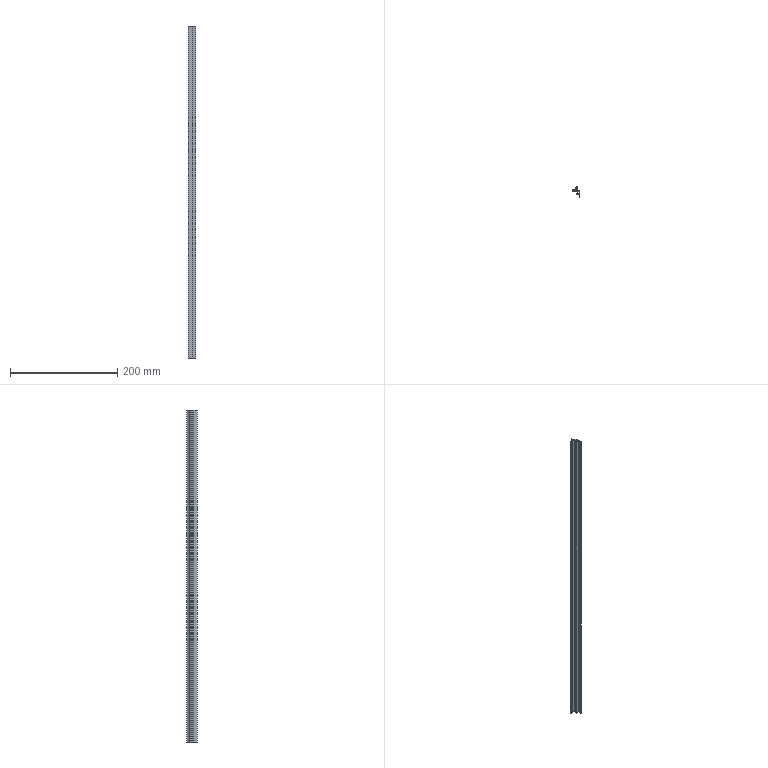Part | SolidWorks | features BaseBody 1, ICE 1, MoveFace 1 | 1 solid | 27 faces | box 14 x 20.3 x 620 mm | volume 31568 mm3 | plane 20 | cylinder 7 | commonest cylinder face diameters 0.387 x2 0.8 x2 0.4 x1 20 x1 22 x1
STEP:
#1=CARTESIAN_POINT('',(-5.304,-0.625,200.));
#2=VERTEX_POINT('',#1);
#3=CARTESIAN_POINT('',(-5.449,-0.8125,200.));
#4=VERTEX_POINT('',#3);
#5=CARTESIAN_POINT('',(-5.255,-0.8125,200.));
#6=DIRECTION('',(0.,0.,1.));
#7=DIRECTION('',(-1.,0.,0.));
#8=AXIS2_PLACEMENT_3D('',#5,#6,#7);
#9=CIRCLE('',#8,0.1937);
#10=EDGE_CURVE('',#2,#4,#9,.T.);
#11=ORIENTED_EDGE('',*,*,#10,.T.);
#12=CARTESIAN_POINT('',(-5.449,-0.8125,-420.));
#13=VERTEX_POINT('',#12);
#14=CARTESIAN_POINT('',(-5.449,-0.8125,230.));
#15=DIRECTION('',(0.,0.,-1.));
#16=VECTOR('',#15,1000.);
#17=LINE('',#14,#16);
#18=EDGE_CURVE('',#4,#13,#17,.T.);
#19=ORIENTED_EDGE('',*,*,#18,.T.);
#20=CARTESIAN_POINT('',(-5.304,-0.625,-420.));
#21=VERTEX_POINT('',#20);
#22=CARTESIAN_POINT('',(-5.255,-0.8125,-420.));
#23=DIRECTION('',(0.,0.,-1.));
#24=DIRECTION('',(1.,0.,0.));
#25=AXIS2_PLACEMENT_3D('',#22,#23,#24);
#26=CIRCLE('',#25,0.1937);
#27=EDGE_CURVE('',#13,#21,#26,.T.);
#28=ORIENTED_EDGE('',*,*,#27,.T.);
#29=CARTESIAN_POINT('',(-5.304,-0.625,230.));
#30=DIRECTION('',(0.,0.,-1.));
#31=VECTOR('',#30,1000.);
#32=LINE('',#29,#31);
#33=EDGE_CURVE('',#2,#21,#32,.T.);
#34=ORIENTED_EDGE('',*,*,#33,.F.);
#35=EDGE_LOOP('',(#11,#19,#28,#34));
#36=FACE_OUTER_BOUND('',#35,.T.);
#37=CARTESIAN_POINT('',(-5.255,-0.8125,230.));
#38=DIRECTION('',(0.,0.,-1.));
#39=DIRECTION('',(-1.,0.,0.));
#40=AXIS2_PLACEMENT_3D('',#37,#38,#39);
#41=CYLINDRICAL_SURFACE('',#40,0.1937);
#42=ADVANCED_FACE('',(#36),#41,.F.);
#43=CARTESIAN_POINT('',(5.,-1.,-420.));
#44=VERTEX_POINT('',#43);
#45=CARTESIAN_POINT('',(5.,-14.3,-420.));
#46=VERTEX_POINT('',#45);
#47=CARTESIAN_POINT('',(5.,29.623,-420.));
#48=DIRECTION('',(0.,-1.,0.));
#49=VECTOR('',#48,1000.);
#50=LINE('',#47,#49);
#51=EDGE_CURVE('',#44,#46,#50,.T.);
#52=ORIENTED_EDGE('',*,*,#51,.F.);
#53=CARTESIAN_POINT('',(5.,-1.,200.));
#54=VERTEX_POINT('',#53);
#55=CARTESIAN_POINT('',(5.,-1.,230.));
#56=DIRECTION('',(0.,0.,-1.));
#57=VECTOR('',#56,1000.);
#58=LINE('',#55,#57);
#59=EDGE_CURVE('',#54,#44,#58,.T.);
#60=ORIENTED_EDGE('',*,*,#59,.F.);
#61=CARTESIAN_POINT('',(5.,-14.3,200.));
#62=VERTEX_POINT('',#61);
#63=CARTESIAN_POINT('',(5.,-14.3,200.));
#64=DIRECTION('',(0.,1.,0.));
#65=VECTOR('',#64,1000.);
#66=LINE('',#63,#65);
#67=EDGE_CURVE('',#62,#54,#66,.T.);
#68=ORIENTED_EDGE('',*,*,#67,.F.);
#69=CARTESIAN_POINT('',(5.,-14.3,230.));
#70=DIRECTION('',(0.,0.,1.));
#71=VECTOR('',#70,1000.);
#72=LINE('',#69,#71);
#73=EDGE_CURVE('',#46,#62,#72,.T.);
#74=ORIENTED_EDGE('',*,*,#73,.F.);
#75=EDGE_LOOP('',(#52,#60,#68,#74));
#76=FACE_OUTER_BOUND('',#75,.T.);
#77=CARTESIAN_POINT('',(5.,-14.3,230.));
#78=DIRECTION('',(-1.,0.,0.));
#79=DIRECTION('',(0.,0.,1.));
#80=AXIS2_PLACEMENT_3D('',#77,#78,#79);
#81=PLANE('',#80);
#82=ADVANCED_FACE('',(#76),#81,.F.);
#83=CARTESIAN_POINT('',(-9.,-2.,-420.));
#84=VERTEX_POINT('',#83);
#85=CARTESIAN_POINT('',(-9.,-2.,200.));
#86=VERTEX_POINT('',#85);
#87=CARTESIAN_POINT('',(-9.,-2.,230.));
#88=DIRECTION('',(0.,0.,1.));
#89=VECTOR('',#88,1000.);
#90=LINE('',#87,#89);
#91=EDGE_CURVE('',#84,#86,#90,.T.);
#92=ORIENTED_EDGE('',*,*,#91,.F.);
#93=CARTESIAN_POINT('',(0.9,-2.,-420.));
#94=VERTEX_POINT('',#93);
#95=CARTESIAN_POINT('',(5.,-2.,-420.));
#96=DIRECTION('',(-1.,0.,0.));
#97=VECTOR('',#96,1000.);
#98=LINE('',#95,#97);
#99=EDGE_CURVE('',#94,#84,#98,.T.);
#100=ORIENTED_EDGE('',*,*,#99,.F.);
#101=CARTESIAN_POINT('',(0.9,-2.,200.));
#102=VERTEX_POINT('',#101);
#103=CARTESIAN_POINT('',(0.9,-2.,230.));
#104=DIRECTION('',(0.,0.,-1.));
#105=VECTOR('',#104,1000.);
#106=LINE('',#103,#105);
#107=EDGE_CURVE('',#102,#94,#106,.T.);
#108=ORIENTED_EDGE('',*,*,#107,.F.);
#109=CARTESIAN_POINT('',(5.,-2.,200.));
#110=DIRECTION('',(1.,0.,0.));
#111=VECTOR('',#110,1000.);
#112=LINE('',#109,#111);
#113=EDGE_CURVE('',#86,#102,#112,.T.);
#114=ORIENTED_EDGE('',*,*,#113,.F.);
#115=EDGE_LOOP('',(#92,#100,#108,#114));
#116=FACE_OUTER_BOUND('',#115,.T.);
#117=CARTESIAN_POINT('',(-9.,-2.,230.));
#118=DIRECTION('',(0.,1.,0.));
#119=DIRECTION('',(0.,0.,1.));
#120=AXIS2_PLACEMENT_3D('',#117,#118,#119);
#121=PLANE('',#120);
#122=ADVANCED_FACE('',(#116),#121,.F.);
#123=CARTESIAN_POINT('',(4.,-6.,200.));
#124=VERTEX_POINT('',#123);
#125=CARTESIAN_POINT('',(4.,-3.,200.));
#126=VERTEX_POINT('',#125);
#127=CARTESIAN_POINT('',(4.,29.623,200.));
#128=DIRECTION('',(0.,1.,0.));
#129=VECTOR('',#128,1000.);
#130=LINE('',#127,#129);
#131=EDGE_CURVE('',#124,#126,#130,.T.);
#132=ORIENTED_EDGE('',*,*,#131,.F.);
#133=CARTESIAN_POINT('',(1.,-6.,200.));
#134=VERTEX_POINT('',#133);
#135=CARTESIAN_POINT('',(5.,-6.,200.));
#136=DIRECTION('',(1.,0.,0.));
#137=VECTOR('',#136,1000.);
#138=LINE('',#135,#137);
#139=EDGE_CURVE('',#134,#124,#138,.T.);
#140=ORIENTED_EDGE('',*,*,#139,.F.);
#141=CARTESIAN_POINT('',(1.,-6.7,200.));
#142=VERTEX_POINT('',#141);
#143=CARTESIAN_POINT('',(1.,-6.,200.));
#144=DIRECTION('',(0.,-1.,0.));
#145=VECTOR('',#144,1000.);
#146=LINE('',#143,#145);
#147=EDGE_CURVE('',#134,#142,#146,.T.);
#148=ORIENTED_EDGE('',*,*,#147,.T.);
#149=CARTESIAN_POINT('',(-1.7,-6.7,200.));
#150=VERTEX_POINT('',#149);
#151=CARTESIAN_POINT('',(5.,-6.7,200.));
#152=DIRECTION('',(1.,0.,0.));
#153=VECTOR('',#152,1000.);
#154=LINE('',#151,#153);
#155=EDGE_CURVE('',#150,#142,#154,.T.);
#156=ORIENTED_EDGE('',*,*,#155,.F.);
#157=CARTESIAN_POINT('',(-1.7,-7.7,200.));
#158=VERTEX_POINT('',#157);
#159=CARTESIAN_POINT('',(-1.7,-6.7,200.));
#160=DIRECTION('',(0.,-1.,0.));
#161=VECTOR('',#160,1000.);
#162=LINE('',#159,#161);
#163=EDGE_CURVE('',#150,#158,#162,.T.);
#164=ORIENTED_EDGE('',*,*,#163,.T.);
#165=CARTESIAN_POINT('',(4.,-7.7,200.));
#166=VERTEX_POINT('',#165);
#167=CARTESIAN_POINT('',(5.,-7.7,200.));
#168=DIRECTION('',(-1.,0.,0.));
#169=VECTOR('',#168,1000.);
#170=LINE('',#167,#169);
#171=EDGE_CURVE('',#166,#158,#170,.T.);
#172=ORIENTED_EDGE('',*,*,#171,.F.);
#173=CARTESIAN_POINT('',(4.,-14.3,200.));
#174=VERTEX_POINT('',#173);
#175=CARTESIAN_POINT('',(4.,29.623,200.));
#176=DIRECTION('',(0.,1.,0.));
#177=VECTOR('',#176,1000.);
#178=LINE('',#175,#177);
#179=EDGE_CURVE('',#174,#166,#178,.T.);
#180=ORIENTED_EDGE('',*,*,#179,.F.);
#181=CARTESIAN_POINT('',(5.,-14.3,200.));
#182=DIRECTION('',(-1.,0.,0.));
#183=VECTOR('',#182,1000.);
#184=LINE('',#181,#183);
#185=EDGE_CURVE('',#62,#174,#184,.T.);
#186=ORIENTED_EDGE('',*,*,#185,.F.);
#187=ORIENTED_EDGE('',*,*,#67,.T.);
#188=CARTESIAN_POINT('',(-5.207,-1.,200.));
#189=VERTEX_POINT('',#188);
#190=CARTESIAN_POINT('',(5.,-1.,200.));
#191=DIRECTION('',(1.,0.,0.));
#192=VECTOR('',#191,1000.);
#193=LINE('',#190,#192);
#194=EDGE_CURVE('',#189,#54,#193,.T.);
#195=ORIENTED_EDGE('',*,*,#194,.F.);
#196=CARTESIAN_POINT('',(-5.255,-0.8125,200.));
#197=DIRECTION('',(0.,0.,1.));
#198=DIRECTION('',(-1.,0.,0.));
#199=AXIS2_PLACEMENT_3D('',#196,#197,#198);
#200=CIRCLE('',#199,0.1937);
#201=EDGE_CURVE('',#4,#189,#200,.T.);
#202=ORIENTED_EDGE('',*,*,#201,.F.);
#203=ORIENTED_EDGE('',*,*,#10,.F.);
#204=CARTESIAN_POINT('',(-1.368,3.063,200.));
#205=VERTEX_POINT('',#204);
#206=CARTESIAN_POINT('',(-10.628,9.,200.));
#207=DIRECTION('',(0.,0.,1.));
#208=DIRECTION('',(-1.,0.,0.));
#209=AXIS2_PLACEMENT_3D('',#206,#207,#208);
#210=CIRCLE('',#209,11.);
#211=EDGE_CURVE('',#2,#205,#210,.T.);
#212=ORIENTED_EDGE('',*,*,#211,.T.);
#213=CARTESIAN_POINT('',(-1.,2.955,200.));
#214=VERTEX_POINT('',#213);
#215=CARTESIAN_POINT('',(-1.2,2.955,200.));
#216=DIRECTION('',(0.,0.,1.));
#217=DIRECTION('',(-1.,0.,0.));
#218=AXIS2_PLACEMENT_3D('',#215,#216,#217);
#219=CIRCLE('',#218,0.2);
#220=EDGE_CURVE('',#214,#205,#219,.T.);
#221=ORIENTED_EDGE('',*,*,#220,.F.);
#222=CARTESIAN_POINT('',(-1.,1.5,200.));
#223=VERTEX_POINT('',#222);
#224=CARTESIAN_POINT('',(-1.,2.955,200.));
#225=DIRECTION('',(0.,1.,0.));
#226=VECTOR('',#225,1000.);
#227=LINE('',#224,#226);
#228=EDGE_CURVE('',#223,#214,#227,.T.);
#229=ORIENTED_EDGE('',*,*,#228,.F.);
#230=CARTESIAN_POINT('',(0.,1.5,200.));
#231=VERTEX_POINT('',#230);
#232=CARTESIAN_POINT('',(-1.,1.5,200.));
#233=DIRECTION('',(-1.,0.,0.));
#234=VECTOR('',#233,1000.);
#235=LINE('',#232,#234);
#236=EDGE_CURVE('',#231,#223,#235,.T.);
#237=ORIENTED_EDGE('',*,*,#236,.F.);
#238=CARTESIAN_POINT('',(0.,6.,200.));
#239=VERTEX_POINT('',#238);
#240=CARTESIAN_POINT('',(0.,1.5,200.));
#241=DIRECTION('',(0.,-1.,0.));
#242=VECTOR('',#241,1000.);
#243=LINE('',#240,#242);
#244=EDGE_CURVE('',#239,#231,#243,.T.);
#245=ORIENTED_EDGE('',*,*,#244,.F.);
#246=CARTESIAN_POINT('',(-0.8,6.,200.));
#247=VERTEX_POINT('',#246);
#248=CARTESIAN_POINT('',(0.,6.,200.));
#249=DIRECTION('',(1.,0.,0.));
#250=VECTOR('',#249,1000.);
#251=LINE('',#248,#250);
#252=EDGE_CURVE('',#247,#239,#251,.T.);
#253=ORIENTED_EDGE('',*,*,#252,.F.);
#254=CARTESIAN_POINT('',(-1.178,5.731,200.));
#255=VERTEX_POINT('',#254);
#256=CARTESIAN_POINT('',(-0.8,5.6,200.));
#257=DIRECTION('',(0.,0.,1.));
#258=DIRECTION('',(-1.,0.,0.));
#259=AXIS2_PLACEMENT_3D('',#256,#257,#258);
#260=CIRCLE('',#259,0.4);
#261=EDGE_CURVE('',#247,#255,#260,.T.);
#262=ORIENTED_EDGE('',*,*,#261,.T.);
#263=CARTESIAN_POINT('',(-8.678,-0.8077,200.));
#264=VERTEX_POINT('',#263);
#265=CARTESIAN_POINT('',(-10.628,9.,200.));
#266=DIRECTION('',(0.,0.,1.));
#267=DIRECTION('',(-1.,0.,0.));
#268=AXIS2_PLACEMENT_3D('',#265,#266,#267);
#269=CIRCLE('',#268,10.);
#270=EDGE_CURVE('',#264,#255,#269,.T.);
#271=ORIENTED_EDGE('',*,*,#270,.F.);
#272=CARTESIAN_POINT('',(-9.,-1.2,200.));
#273=VERTEX_POINT('',#272);
#274=CARTESIAN_POINT('',(-8.6,-1.2,200.));
#275=DIRECTION('',(0.,0.,1.));
#276=DIRECTION('',(-1.,0.,0.));
#277=AXIS2_PLACEMENT_3D('',#274,#275,#276);
#278=CIRCLE('',#277,0.4);
#279=EDGE_CURVE('',#264,#273,#278,.T.);
#280=ORIENTED_EDGE('',*,*,#279,.T.);
#281=CARTESIAN_POINT('',(-9.,8.,200.));
#282=DIRECTION('',(0.,-1.,0.));
#283=VECTOR('',#282,1000.);
#284=LINE('',#281,#283);
#285=EDGE_CURVE('',#273,#86,#284,.T.);
#286=ORIENTED_EDGE('',*,*,#285,.T.);
#287=ORIENTED_EDGE('',*,*,#113,.T.);
#288=CARTESIAN_POINT('',(0.9,-3.,200.));
#289=VERTEX_POINT('',#288);
#290=CARTESIAN_POINT('',(0.9,29.623,200.));
#291=DIRECTION('',(0.,1.,0.));
#292=VECTOR('',#291,1000.);
#293=LINE('',#290,#292);
#294=EDGE_CURVE('',#289,#102,#293,.T.);
#295=ORIENTED_EDGE('',*,*,#294,.F.);
#296=CARTESIAN_POINT('',(5.,-3.,200.));
#297=DIRECTION('',(-1.,0.,0.));
#298=VECTOR('',#297,1000.);
#299=LINE('',#296,#298);
#300=EDGE_CURVE('',#126,#289,#299,.T.);
#301=ORIENTED_EDGE('',*,*,#300,.F.);
#302=EDGE_LOOP('',(#132,#140,#148,#156,#164,#172,#180,#186,#187,#195,#202,#203,#212,#221,#229,#237,#245,#253,#262,#271,#280,#286,#287,#295,#301));
#303=FACE_OUTER_BOUND('',#302,.T.);
#304=CARTESIAN_POINT('',(5.,29.623,200.));
#305=DIRECTION('',(0.,0.,-1.));
#306=DIRECTION('',(-1.,0.,0.));
#307=AXIS2_PLACEMENT_3D('',#304,#305,#306);
#308=PLANE('',#307);
#309=ADVANCED_FACE('',(#303),#308,.F.);
#310=ORIENTED_EDGE('',*,*,#185,.T.);
#311=CARTESIAN_POINT('',(4.,-14.3,-420.));
#312=VERTEX_POINT('',#311);
#313=CARTESIAN_POINT('',(4.,-14.3,230.));
#314=DIRECTION('',(0.,0.,1.));
#315=VECTOR('',#314,1000.);
#316=LINE('',#313,#315);
#317=EDGE_CURVE('',#312,#174,#316,.T.);
#318=ORIENTED_EDGE('',*,*,#317,.F.);
#319=CARTESIAN_POINT('',(5.,-14.3,-420.));
#320=DIRECTION('',(-1.,0.,0.));
#321=VECTOR('',#320,1000.);
#322=LINE('',#319,#321);
#323=EDGE_CURVE('',#46,#312,#322,.T.);
#324=ORIENTED_EDGE('',*,*,#323,.F.);
#325=ORIENTED_EDGE('',*,*,#73,.T.);
#326=EDGE_LOOP('',(#310,#318,#324,#325));
#327=FACE_OUTER_BOUND('',#326,.T.);
#328=CARTESIAN_POINT('',(4.,-14.3,230.));
#329=DIRECTION('',(0.,1.,0.));
#330=DIRECTION('',(0.,0.,1.));
#331=AXIS2_PLACEMENT_3D('',#328,#329,#330);
#332=PLANE('',#331);
#333=ADVANCED_FACE('',(#327),#332,.F.);
#334=ORIENTED_EDGE('',*,*,#51,.T.);
#335=ORIENTED_EDGE('',*,*,#323,.T.);
#336=CARTESIAN_POINT('',(4.,-7.7,-420.));
#337=VERTEX_POINT('',#336);
#338=CARTESIAN_POINT('',(4.,-7.7,-420.));
#339=DIRECTION('',(0.,-1.,0.));
#340=VECTOR('',#339,1000.);
#341=LINE('',#338,#340);
#342=EDGE_CURVE('',#337,#312,#341,.T.);
#343=ORIENTED_EDGE('',*,*,#342,.F.);
#344=CARTESIAN_POINT('',(-1.7,-7.7,-420.));
#345=VERTEX_POINT('',#344);
#346=CARTESIAN_POINT('',(-1.7,-7.7,-420.));
#347=DIRECTION('',(1.,0.,0.));
#348=VECTOR('',#347,1000.);
#349=LINE('',#346,#348);
#350=EDGE_CURVE('',#345,#337,#349,.T.);
#351=ORIENTED_EDGE('',*,*,#350,.F.);
#352=CARTESIAN_POINT('',(-1.7,-6.7,-420.));
#353=VERTEX_POINT('',#352);
#354=CARTESIAN_POINT('',(-1.7,29.623,-420.));
#355=DIRECTION('',(0.,1.,0.));
#356=VECTOR('',#355,1000.);
#357=LINE('',#354,#356);
#358=EDGE_CURVE('',#345,#353,#357,.T.);
#359=ORIENTED_EDGE('',*,*,#358,.T.);
#360=CARTESIAN_POINT('',(1.,-6.7,-420.));
#361=VERTEX_POINT('',#360);
#362=CARTESIAN_POINT('',(1.,-6.7,-420.));
#363=DIRECTION('',(-1.,0.,0.));
#364=VECTOR('',#363,1000.);
#365=LINE('',#362,#364);
#366=EDGE_CURVE('',#361,#353,#365,.T.);
#367=ORIENTED_EDGE('',*,*,#366,.F.);
#368=CARTESIAN_POINT('',(1.,-6.,-420.));
#369=VERTEX_POINT('',#368);
#370=CARTESIAN_POINT('',(1.,29.623,-420.));
#371=DIRECTION('',(0.,1.,0.));
#372=VECTOR('',#371,1000.);
#373=LINE('',#370,#372);
#374=EDGE_CURVE('',#361,#369,#373,.T.);
#375=ORIENTED_EDGE('',*,*,#374,.T.);
#376=CARTESIAN_POINT('',(4.,-6.,-420.));
#377=VERTEX_POINT('',#376);
#378=CARTESIAN_POINT('',(4.,-6.,-420.));
#379=DIRECTION('',(-1.,0.,0.));
#380=VECTOR('',#379,1000.);
#381=LINE('',#378,#380);
#382=EDGE_CURVE('',#377,#369,#381,.T.);
#383=ORIENTED_EDGE('',*,*,#382,.F.);
#384=CARTESIAN_POINT('',(4.,-3.,-420.));
#385=VERTEX_POINT('',#384);
#386=CARTESIAN_POINT('',(4.,-3.,-420.));
#387=DIRECTION('',(0.,-1.,0.));
#388=VECTOR('',#387,1000.);
#389=LINE('',#386,#388);
#390=EDGE_CURVE('',#385,#377,#389,.T.);
#391=ORIENTED_EDGE('',*,*,#390,.F.);
#392=CARTESIAN_POINT('',(0.9,-3.,-420.));
#393=VERTEX_POINT('',#392);
#394=CARTESIAN_POINT('',(0.9,-3.,-420.));
#395=DIRECTION('',(1.,0.,0.));
#396=VECTOR('',#395,1000.);
#397=LINE('',#394,#396);
#398=EDGE_CURVE('',#393,#385,#397,.T.);
#399=ORIENTED_EDGE('',*,*,#398,.F.);
#400=CARTESIAN_POINT('',(0.9,-2.,-420.));
#401=DIRECTION('',(0.,-1.,0.));
#402=VECTOR('',#401,1000.);
#403=LINE('',#400,#402);
#404=EDGE_CURVE('',#94,#393,#403,.T.);
#405=ORIENTED_EDGE('',*,*,#404,.F.);
#406=ORIENTED_EDGE('',*,*,#99,.T.);
#407=CARTESIAN_POINT('',(-9.,-1.2,-420.));
#408=VERTEX_POINT('',#407);
#409=CARTESIAN_POINT('',(-9.,-1.2,-420.));
#410=DIRECTION('',(0.,-1.,0.));
#411=VECTOR('',#410,1000.);
#412=LINE('',#409,#411);
#413=EDGE_CURVE('',#408,#84,#412,.T.);
#414=ORIENTED_EDGE('',*,*,#413,.F.);
#415=CARTESIAN_POINT('',(-8.678,-0.8077,-420.));
#416=VERTEX_POINT('',#415);
#417=CARTESIAN_POINT('',(-8.6,-1.2,-420.));
#418=DIRECTION('',(0.,0.,-1.));
#419=DIRECTION('',(1.,0.,0.));
#420=AXIS2_PLACEMENT_3D('',#417,#418,#419);
#421=CIRCLE('',#420,0.4);
#422=EDGE_CURVE('',#408,#416,#421,.T.);
#423=ORIENTED_EDGE('',*,*,#422,.T.);
#424=CARTESIAN_POINT('',(-1.178,5.731,-420.));
#425=VERTEX_POINT('',#424);
#426=CARTESIAN_POINT('',(-10.628,9.,-420.));
#427=DIRECTION('',(0.,0.,-1.));
#428=DIRECTION('',(1.,0.,0.));
#429=AXIS2_PLACEMENT_3D('',#426,#427,#428);
#430=CIRCLE('',#429,10.);
#431=EDGE_CURVE('',#425,#416,#430,.T.);
#432=ORIENTED_EDGE('',*,*,#431,.F.);
#433=CARTESIAN_POINT('',(-0.8,6.,-420.));
#434=VERTEX_POINT('',#433);
#435=CARTESIAN_POINT('',(-0.8,5.6,-420.));
#436=DIRECTION('',(0.,0.,-1.));
#437=DIRECTION('',(1.,0.,0.));
#438=AXIS2_PLACEMENT_3D('',#435,#436,#437);
#439=CIRCLE('',#438,0.4);
#440=EDGE_CURVE('',#425,#434,#439,.T.);
#441=ORIENTED_EDGE('',*,*,#440,.T.);
#442=CARTESIAN_POINT('',(0.,6.,-420.));
#443=VERTEX_POINT('',#442);
#444=CARTESIAN_POINT('',(0.,6.,-420.));
#445=DIRECTION('',(-1.,0.,0.));
#446=VECTOR('',#445,1000.);
#447=LINE('',#444,#446);
#448=EDGE_CURVE('',#443,#434,#447,.T.);
#449=ORIENTED_EDGE('',*,*,#448,.F.);
#450=CARTESIAN_POINT('',(0.,1.5,-420.));
#451=VERTEX_POINT('',#450);
#452=CARTESIAN_POINT('',(0.,1.5,-420.));
#453=DIRECTION('',(0.,1.,0.));
#454=VECTOR('',#453,1000.);
#455=LINE('',#452,#454);
#456=EDGE_CURVE('',#451,#443,#455,.T.);
#457=ORIENTED_EDGE('',*,*,#456,.F.);
#458=CARTESIAN_POINT('',(-1.,1.5,-420.));
#459=VERTEX_POINT('',#458);
#460=CARTESIAN_POINT('',(-1.,1.5,-420.));
#461=DIRECTION('',(1.,0.,0.));
#462=VECTOR('',#461,1000.);
#463=LINE('',#460,#462);
#464=EDGE_CURVE('',#459,#451,#463,.T.);
#465=ORIENTED_EDGE('',*,*,#464,.F.);
#466=CARTESIAN_POINT('',(-1.,2.955,-420.));
#467=VERTEX_POINT('',#466);
#468=CARTESIAN_POINT('',(-1.,2.955,-420.));
#469=DIRECTION('',(0.,-1.,0.));
#470=VECTOR('',#469,1000.);
#471=LINE('',#468,#470);
#472=EDGE_CURVE('',#467,#459,#471,.T.);
#473=ORIENTED_EDGE('',*,*,#472,.F.);
#474=CARTESIAN_POINT('',(-1.368,3.063,-420.));
#475=VERTEX_POINT('',#474);
#476=CARTESIAN_POINT('',(-1.2,2.955,-420.));
#477=DIRECTION('',(0.,0.,-1.));
#478=DIRECTION('',(1.,0.,0.));
#479=AXIS2_PLACEMENT_3D('',#476,#477,#478);
#480=CIRCLE('',#479,0.2);
#481=EDGE_CURVE('',#475,#467,#480,.T.);
#482=ORIENTED_EDGE('',*,*,#481,.F.);
#483=CARTESIAN_POINT('',(-10.628,9.,-420.));
#484=DIRECTION('',(0.,0.,-1.));
#485=DIRECTION('',(1.,0.,0.));
#486=AXIS2_PLACEMENT_3D('',#483,#484,#485);
#487=CIRCLE('',#486,11.);
#488=EDGE_CURVE('',#475,#21,#487,.T.);
#489=ORIENTED_EDGE('',*,*,#488,.T.);
#490=ORIENTED_EDGE('',*,*,#27,.F.);
#491=CARTESIAN_POINT('',(-5.207,-1.,-420.));
#492=VERTEX_POINT('',#491);
#493=CARTESIAN_POINT('',(-5.255,-0.8125,-420.));
#494=DIRECTION('',(0.,0.,-1.));
#495=DIRECTION('',(1.,0.,0.));
#496=AXIS2_PLACEMENT_3D('',#493,#494,#495);
#497=CIRCLE('',#496,0.1937);
#498=EDGE_CURVE('',#492,#13,#497,.T.);
#499=ORIENTED_EDGE('',*,*,#498,.F.);
#500=CARTESIAN_POINT('',(5.,-1.,-420.));
#501=DIRECTION('',(-1.,0.,0.));
#502=VECTOR('',#501,1000.);
#503=LINE('',#500,#502);
#504=EDGE_CURVE('',#44,#492,#503,.T.);
#505=ORIENTED_EDGE('',*,*,#504,.F.);
#506=EDGE_LOOP('',(#334,#335,#343,#351,#359,#367,#375,#383,#391,#399,#405,#406,#414,#423,#432,#441,#449,#457,#465,#473,#482,#489,#490,#499,#505));
#507=FACE_OUTER_BOUND('',#506,.T.);
#508=CARTESIAN_POINT('',(5.,29.623,-420.));
#509=DIRECTION('',(0.,0.,1.));
#510=DIRECTION('',(1.,0.,0.));
#511=AXIS2_PLACEMENT_3D('',#508,#509,#510);
#512=PLANE('',#511);
#513=ADVANCED_FACE('',(#507),#512,.F.);
#514=ORIENTED_EDGE('',*,*,#59,.T.);
#515=ORIENTED_EDGE('',*,*,#504,.T.);
#516=CARTESIAN_POINT('',(-5.207,-1.,230.));
#517=DIRECTION('',(0.,0.,-1.));
#518=VECTOR('',#517,1000.);
#519=LINE('',#516,#518);
#520=EDGE_CURVE('',#189,#492,#519,.T.);
#521=ORIENTED_EDGE('',*,*,#520,.F.);
#522=ORIENTED_EDGE('',*,*,#194,.T.);
#523=EDGE_LOOP('',(#514,#515,#521,#522));
#524=FACE_OUTER_BOUND('',#523,.T.);
#525=CARTESIAN_POINT('',(5.,-1.,230.));
#526=DIRECTION('',(0.,-1.,0.));
#527=DIRECTION('',(0.,0.,-1.));
#528=AXIS2_PLACEMENT_3D('',#525,#526,#527);
#529=PLANE('',#528);
#530=ADVANCED_FACE('',(#524),#529,.F.);
#531=CARTESIAN_POINT('',(-9.,-1.2,230.));
#532=DIRECTION('',(0.,0.,1.));
#533=VECTOR('',#532,1000.);
#534=LINE('',#531,#533);
#535=EDGE_CURVE('',#408,#273,#534,.T.);
#536=ORIENTED_EDGE('',*,*,#535,.F.);
#537=ORIENTED_EDGE('',*,*,#413,.T.);
#538=ORIENTED_EDGE('',*,*,#91,.T.);
#539=ORIENTED_EDGE('',*,*,#285,.F.);
#540=EDGE_LOOP('',(#536,#537,#538,#539));
#541=FACE_OUTER_BOUND('',#540,.T.);
#542=CARTESIAN_POINT('',(-9.,-1.2,230.));
#543=DIRECTION('',(1.,0.,0.));
#544=DIRECTION('',(0.,0.,-1.));
#545=AXIS2_PLACEMENT_3D('',#542,#543,#544);
#546=PLANE('',#545);
#547=ADVANCED_FACE('',(#541),#546,.F.);
#548=ORIENTED_EDGE('',*,*,#294,.T.);
#549=ORIENTED_EDGE('',*,*,#107,.T.);
#550=ORIENTED_EDGE('',*,*,#404,.T.);
#551=CARTESIAN_POINT('',(0.9,-3.,230.));
#552=DIRECTION('',(0.,0.,-1.));
#553=VECTOR('',#552,1000.);
#554=LINE('',#551,#553);
#555=EDGE_CURVE('',#289,#393,#554,.T.);
#556=ORIENTED_EDGE('',*,*,#555,.F.);
#557=EDGE_LOOP('',(#548,#549,#550,#556));
#558=FACE_OUTER_BOUND('',#557,.T.);
#559=CARTESIAN_POINT('',(0.9,-2.,230.));
#560=DIRECTION('',(1.,0.,0.));
#561=DIRECTION('',(0.,0.,-1.));
#562=AXIS2_PLACEMENT_3D('',#559,#560,#561);
#563=PLANE('',#562);
#564=ADVANCED_FACE('',(#558),#563,.F.);
#565=ORIENTED_EDGE('',*,*,#300,.T.);
#566=ORIENTED_EDGE('',*,*,#555,.T.);
#567=ORIENTED_EDGE('',*,*,#398,.T.);
#568=CARTESIAN_POINT('',(4.,-3.,230.));
#569=DIRECTION('',(0.,0.,-1.));
#570=VECTOR('',#569,1000.);
#571=LINE('',#568,#570);
#572=EDGE_CURVE('',#126,#385,#571,.T.);
#573=ORIENTED_EDGE('',*,*,#572,.F.);
#574=EDGE_LOOP('',(#565,#566,#567,#573));
#575=FACE_OUTER_BOUND('',#574,.T.);
#576=CARTESIAN_POINT('',(0.9,-3.,230.));
#577=DIRECTION('',(0.,1.,0.));
#578=DIRECTION('',(0.,0.,1.));
#579=AXIS2_PLACEMENT_3D('',#576,#577,#578);
#580=PLANE('',#579);
#581=ADVANCED_FACE('',(#575),#580,.F.);
#582=ORIENTED_EDGE('',*,*,#131,.T.);
#583=ORIENTED_EDGE('',*,*,#572,.T.);
#584=ORIENTED_EDGE('',*,*,#390,.T.);
#585=CARTESIAN_POINT('',(4.,-6.,230.));
#586=DIRECTION('',(0.,0.,-1.));
#587=VECTOR('',#586,1000.);
#588=LINE('',#585,#587);
#589=EDGE_CURVE('',#124,#377,#588,.T.);
#590=ORIENTED_EDGE('',*,*,#589,.F.);
#591=EDGE_LOOP('',(#582,#583,#584,#590));
#592=FACE_OUTER_BOUND('',#591,.T.);
#593=CARTESIAN_POINT('',(4.,-3.,230.));
#594=DIRECTION('',(1.,0.,0.));
#595=DIRECTION('',(0.,0.,-1.));
#596=AXIS2_PLACEMENT_3D('',#593,#594,#595);
#597=PLANE('',#596);
#598=ADVANCED_FACE('',(#592),#597,.F.);
#599=ORIENTED_EDGE('',*,*,#139,.T.);
#600=ORIENTED_EDGE('',*,*,#589,.T.);
#601=ORIENTED_EDGE('',*,*,#382,.T.);
#602=CARTESIAN_POINT('',(1.,-6.,230.));
#603=DIRECTION('',(0.,0.,-1.));
#604=VECTOR('',#603,1000.);
#605=LINE('',#602,#604);
#606=EDGE_CURVE('',#134,#369,#605,.T.);
#607=ORIENTED_EDGE('',*,*,#606,.F.);
#608=EDGE_LOOP('',(#599,#600,#601,#607));
#609=FACE_OUTER_BOUND('',#608,.T.);
#610=CARTESIAN_POINT('',(4.,-6.,230.));
#611=DIRECTION('',(0.,-1.,0.));
#612=DIRECTION('',(0.,0.,-1.));
#613=AXIS2_PLACEMENT_3D('',#610,#611,#612);
#614=PLANE('',#613);
#615=ADVANCED_FACE('',(#609),#614,.F.);
#616=ORIENTED_EDGE('',*,*,#155,.T.);
#617=CARTESIAN_POINT('',(1.,-6.7,230.));
#618=DIRECTION('',(0.,0.,1.));
#619=VECTOR('',#618,1000.);
#620=LINE('',#617,#619);
#621=EDGE_CURVE('',#361,#142,#620,.T.);
#622=ORIENTED_EDGE('',*,*,#621,.F.);
#623=ORIENTED_EDGE('',*,*,#366,.T.);
#624=CARTESIAN_POINT('',(-1.7,-6.7,230.));
#625=DIRECTION('',(0.,0.,-1.));
#626=VECTOR('',#625,1000.);
#627=LINE('',#624,#626);
#628=EDGE_CURVE('',#150,#353,#627,.T.);
#629=ORIENTED_EDGE('',*,*,#628,.F.);
#630=EDGE_LOOP('',(#616,#622,#623,#629));
#631=FACE_OUTER_BOUND('',#630,.T.);
#632=CARTESIAN_POINT('',(1.,-6.7,230.));
#633=DIRECTION('',(0.,-1.,0.));
#634=DIRECTION('',(0.,0.,-1.));
#635=AXIS2_PLACEMENT_3D('',#632,#633,#634);
#636=PLANE('',#635);
#637=ADVANCED_FACE('',(#631),#636,.F.);
#638=ORIENTED_EDGE('',*,*,#171,.T.);
#639=CARTESIAN_POINT('',(-1.7,-7.7,230.));
#640=DIRECTION('',(0.,0.,1.));
#641=VECTOR('',#640,1000.);
#642=LINE('',#639,#641);
#643=EDGE_CURVE('',#345,#158,#642,.T.);
#644=ORIENTED_EDGE('',*,*,#643,.F.);
#645=ORIENTED_EDGE('',*,*,#350,.T.);
#646=CARTESIAN_POINT('',(4.,-7.7,230.));
#647=DIRECTION('',(0.,0.,-1.));
#648=VECTOR('',#647,1000.);
#649=LINE('',#646,#648);
#650=EDGE_CURVE('',#166,#337,#649,.T.);
#651=ORIENTED_EDGE('',*,*,#650,.F.);
#652=EDGE_LOOP('',(#638,#644,#645,#651));
#653=FACE_OUTER_BOUND('',#652,.T.);
#654=CARTESIAN_POINT('',(-1.7,-7.7,230.));
#655=DIRECTION('',(0.,1.,0.));
#656=DIRECTION('',(0.,0.,1.));
#657=AXIS2_PLACEMENT_3D('',#654,#655,#656);
#658=PLANE('',#657);
#659=ADVANCED_FACE('',(#653),#658,.F.);
#660=ORIENTED_EDGE('',*,*,#179,.T.);
#661=ORIENTED_EDGE('',*,*,#650,.T.);
#662=ORIENTED_EDGE('',*,*,#342,.T.);
#663=ORIENTED_EDGE('',*,*,#317,.T.);
#664=EDGE_LOOP('',(#660,#661,#662,#663));
#665=FACE_OUTER_BOUND('',#664,.T.);
#666=CARTESIAN_POINT('',(4.,-7.7,230.));
#667=DIRECTION('',(1.,0.,0.));
#668=DIRECTION('',(0.,0.,-1.));
#669=AXIS2_PLACEMENT_3D('',#666,#667,#668);
#670=PLANE('',#669);
#671=ADVANCED_FACE('',(#665),#670,.F.);
#672=ORIENTED_EDGE('',*,*,#18,.F.);
#673=ORIENTED_EDGE('',*,*,#201,.T.);
#674=ORIENTED_EDGE('',*,*,#520,.T.);
#675=ORIENTED_EDGE('',*,*,#498,.T.);
#676=EDGE_LOOP('',(#672,#673,#674,#675));
#677=FACE_OUTER_BOUND('',#676,.T.);
#678=CARTESIAN_POINT('',(-5.255,-0.8125,230.));
#679=DIRECTION('',(0.,0.,-1.));
#680=DIRECTION('',(-1.,0.,0.));
#681=AXIS2_PLACEMENT_3D('',#678,#679,#680);
#682=CYLINDRICAL_SURFACE('',#681,0.1937);
#683=ADVANCED_FACE('',(#677),#682,.F.);
#684=CARTESIAN_POINT('',(-1.,2.955,230.));
#685=DIRECTION('',(0.,0.,1.));
#686=VECTOR('',#685,1000.);
#687=LINE('',#684,#686);
#688=EDGE_CURVE('',#467,#214,#687,.T.);
#689=ORIENTED_EDGE('',*,*,#688,.F.);
#690=ORIENTED_EDGE('',*,*,#472,.T.);
#691=CARTESIAN_POINT('',(-1.,1.5,230.));
#692=DIRECTION('',(0.,0.,-1.));
#693=VECTOR('',#692,1000.);
#694=LINE('',#691,#693);
#695=EDGE_CURVE('',#223,#459,#694,.T.);
#696=ORIENTED_EDGE('',*,*,#695,.F.);
#697=ORIENTED_EDGE('',*,*,#228,.T.);
#698=EDGE_LOOP('',(#689,#690,#696,#697));
#699=FACE_OUTER_BOUND('',#698,.T.);
#700=CARTESIAN_POINT('',(-1.,2.955,230.));
#701=DIRECTION('',(1.,0.,0.));
#702=DIRECTION('',(0.,0.,-1.));
#703=AXIS2_PLACEMENT_3D('',#700,#701,#702);
#704=PLANE('',#703);
#705=ADVANCED_FACE('',(#699),#704,.F.);
#706=ORIENTED_EDGE('',*,*,#488,.F.);
#707=CARTESIAN_POINT('',(-1.368,3.063,230.));
#708=DIRECTION('',(0.,0.,1.));
#709=VECTOR('',#708,1000.);
#710=LINE('',#707,#709);
#711=EDGE_CURVE('',#475,#205,#710,.T.);
#712=ORIENTED_EDGE('',*,*,#711,.T.);
#713=ORIENTED_EDGE('',*,*,#211,.F.);
#714=ORIENTED_EDGE('',*,*,#33,.T.);
#715=EDGE_LOOP('',(#706,#712,#713,#714));
#716=FACE_OUTER_BOUND('',#715,.T.);
#717=CARTESIAN_POINT('',(-10.628,9.,230.));
#718=DIRECTION('',(0.,0.,-1.));
#719=DIRECTION('',(-1.,0.,0.));
#720=AXIS2_PLACEMENT_3D('',#717,#718,#719);
#721=CYLINDRICAL_SURFACE('',#720,11.);
#722=ADVANCED_FACE('',(#716),#721,.T.);
#723=CARTESIAN_POINT('',(-1.178,5.731,230.));
#724=DIRECTION('',(0.,0.,1.));
#725=VECTOR('',#724,1000.);
#726=LINE('',#723,#725);
#727=EDGE_CURVE('',#425,#255,#726,.T.);
#728=ORIENTED_EDGE('',*,*,#727,.F.);
#729=ORIENTED_EDGE('',*,*,#431,.T.);
#730=CARTESIAN_POINT('',(-8.678,-0.8077,230.));
#731=DIRECTION('',(0.,0.,-1.));
#732=VECTOR('',#731,1000.);
#733=LINE('',#730,#732);
#734=EDGE_CURVE('',#264,#416,#733,.T.);
#735=ORIENTED_EDGE('',*,*,#734,.F.);
#736=ORIENTED_EDGE('',*,*,#270,.T.);
#737=EDGE_LOOP('',(#728,#729,#735,#736));
#738=FACE_OUTER_BOUND('',#737,.T.);
#739=CARTESIAN_POINT('',(-10.628,9.,230.));
#740=DIRECTION('',(0.,0.,-1.));
#741=DIRECTION('',(-1.,0.,0.));
#742=AXIS2_PLACEMENT_3D('',#739,#740,#741);
#743=CYLINDRICAL_SURFACE('',#742,10.);
#744=ADVANCED_FACE('',(#738),#743,.F.);
#745=CARTESIAN_POINT('',(0.,1.5,230.));
#746=DIRECTION('',(0.,0.,1.));
#747=VECTOR('',#746,1000.);
#748=LINE('',#745,#747);
#749=EDGE_CURVE('',#451,#231,#748,.T.);
#750=ORIENTED_EDGE('',*,*,#749,.F.);
#751=ORIENTED_EDGE('',*,*,#456,.T.);
#752=CARTESIAN_POINT('',(0.,6.,230.));
#753=DIRECTION('',(0.,0.,-1.));
#754=VECTOR('',#753,1000.);
#755=LINE('',#752,#754);
#756=EDGE_CURVE('',#239,#443,#755,.T.);
#757=ORIENTED_EDGE('',*,*,#756,.F.);
#758=ORIENTED_EDGE('',*,*,#244,.T.);
#759=EDGE_LOOP('',(#750,#751,#757,#758));
#760=FACE_OUTER_BOUND('',#759,.T.);
#761=CARTESIAN_POINT('',(0.,1.5,230.));
#762=DIRECTION('',(-1.,0.,0.));
#763=DIRECTION('',(0.,0.,1.));
#764=AXIS2_PLACEMENT_3D('',#761,#762,#763);
#765=PLANE('',#764);
#766=ADVANCED_FACE('',(#760),#765,.F.);
#767=ORIENTED_EDGE('',*,*,#422,.F.);
#768=ORIENTED_EDGE('',*,*,#535,.T.);
#769=ORIENTED_EDGE('',*,*,#279,.F.);
#770=ORIENTED_EDGE('',*,*,#734,.T.);
#771=EDGE_LOOP('',(#767,#768,#769,#770));
#772=FACE_OUTER_BOUND('',#771,.T.);
#773=CARTESIAN_POINT('',(-8.6,-1.2,230.));
#774=DIRECTION('',(0.,0.,-1.));
#775=DIRECTION('',(-1.,0.,0.));
#776=AXIS2_PLACEMENT_3D('',#773,#774,#775);
#777=CYLINDRICAL_SURFACE('',#776,0.4);
#778=ADVANCED_FACE('',(#772),#777,.T.);
#779=ORIENTED_EDGE('',*,*,#147,.F.);
#780=ORIENTED_EDGE('',*,*,#606,.T.);
#781=ORIENTED_EDGE('',*,*,#374,.F.);
#782=ORIENTED_EDGE('',*,*,#621,.T.);
#783=EDGE_LOOP('',(#779,#780,#781,#782));
#784=FACE_OUTER_BOUND('',#783,.T.);
#785=CARTESIAN_POINT('',(1.,-6.,230.));
#786=DIRECTION('',(1.,0.,0.));
#787=DIRECTION('',(0.,0.,-1.));
#788=AXIS2_PLACEMENT_3D('',#785,#786,#787);
#789=PLANE('',#788);
#790=ADVANCED_FACE('',(#784),#789,.F.);
#791=ORIENTED_EDGE('',*,*,#163,.F.);
#792=ORIENTED_EDGE('',*,*,#628,.T.);
#793=ORIENTED_EDGE('',*,*,#358,.F.);
#794=ORIENTED_EDGE('',*,*,#643,.T.);
#795=EDGE_LOOP('',(#791,#792,#793,#794));
#796=FACE_OUTER_BOUND('',#795,.T.);
#797=CARTESIAN_POINT('',(-1.7,-6.7,230.));
#798=DIRECTION('',(1.,0.,0.));
#799=DIRECTION('',(0.,0.,-1.));
#800=AXIS2_PLACEMENT_3D('',#797,#798,#799);
#801=PLANE('',#800);
#802=ADVANCED_FACE('',(#796),#801,.F.);
#803=ORIENTED_EDGE('',*,*,#711,.F.);
#804=ORIENTED_EDGE('',*,*,#481,.T.);
#805=ORIENTED_EDGE('',*,*,#688,.T.);
#806=ORIENTED_EDGE('',*,*,#220,.T.);
#807=EDGE_LOOP('',(#803,#804,#805,#806));
#808=FACE_OUTER_BOUND('',#807,.T.);
#809=CARTESIAN_POINT('',(-1.2,2.955,230.));
#810=DIRECTION('',(0.,0.,-1.));
#811=DIRECTION('',(-1.,0.,0.));
#812=AXIS2_PLACEMENT_3D('',#809,#810,#811);
#813=CYLINDRICAL_SURFACE('',#812,0.2);
#814=ADVANCED_FACE('',(#808),#813,.F.);
#815=ORIENTED_EDGE('',*,*,#695,.T.);
#816=ORIENTED_EDGE('',*,*,#464,.T.);
#817=ORIENTED_EDGE('',*,*,#749,.T.);
#818=ORIENTED_EDGE('',*,*,#236,.T.);
#819=EDGE_LOOP('',(#815,#816,#817,#818));
#820=FACE_OUTER_BOUND('',#819,.T.);
#821=CARTESIAN_POINT('',(-1.,1.5,230.));
#822=DIRECTION('',(0.,1.,0.));
#823=DIRECTION('',(0.,0.,1.));
#824=AXIS2_PLACEMENT_3D('',#821,#822,#823);
#825=PLANE('',#824);
#826=ADVANCED_FACE('',(#820),#825,.F.);
#827=ORIENTED_EDGE('',*,*,#440,.F.);
#828=ORIENTED_EDGE('',*,*,#727,.T.);
#829=ORIENTED_EDGE('',*,*,#261,.F.);
#830=CARTESIAN_POINT('',(-0.8,6.,230.));
#831=DIRECTION('',(0.,0.,-1.));
#832=VECTOR('',#831,1000.);
#833=LINE('',#830,#832);
#834=EDGE_CURVE('',#247,#434,#833,.T.);
#835=ORIENTED_EDGE('',*,*,#834,.T.);
#836=EDGE_LOOP('',(#827,#828,#829,#835));
#837=FACE_OUTER_BOUND('',#836,.T.);
#838=CARTESIAN_POINT('',(-0.8,5.6,230.));
#839=DIRECTION('',(0.,0.,-1.));
#840=DIRECTION('',(-1.,0.,0.));
#841=AXIS2_PLACEMENT_3D('',#838,#839,#840);
#842=CYLINDRICAL_SURFACE('',#841,0.4);
#843=ADVANCED_FACE('',(#837),#842,.T.);
#844=ORIENTED_EDGE('',*,*,#756,.T.);
#845=ORIENTED_EDGE('',*,*,#448,.T.);
#846=ORIENTED_EDGE('',*,*,#834,.F.);
#847=ORIENTED_EDGE('',*,*,#252,.T.);
#848=EDGE_LOOP('',(#844,#845,#846,#847));
#849=FACE_OUTER_BOUND('',#848,.T.);
#850=CARTESIAN_POINT('',(0.,6.,230.));
#851=DIRECTION('',(0.,-1.,0.));
#852=DIRECTION('',(0.,0.,-1.));
#853=AXIS2_PLACEMENT_3D('',#850,#851,#852);
#854=PLANE('',#853);
#855=ADVANCED_FACE('',(#849),#854,.F.);
#856=CLOSED_SHELL('',(#42,#82,#122,#309,#333,#513,#530,#547,#564,#581,#598,#615,#637,#659,#671,#683,#705,#722,#744,#766,#778,#790,#802,#814,#826,#843,#855));
#857=MANIFOLD_SOLID_BREP('',#856);
#858=CARTESIAN_POINT('',(0.,0.,0.));
#859=DIRECTION('',(0.,0.,1.));
#860=DIRECTION('',(1.,0.,0.));
#861=AXIS2_PLACEMENT_3D('',#858,#859,#860);
#862=(LENGTH_UNIT()NAMED_UNIT(*)SI_UNIT(.MILLI.,.METRE.));
#863=UNCERTAINTY_MEASURE_WITH_UNIT(LENGTH_MEASURE(0.00001),#862,'','');
#864=(NAMED_UNIT(*)PLANE_ANGLE_UNIT()SI_UNIT($,.RADIAN.));
#865=(NAMED_UNIT(*)SI_UNIT($,.STERADIAN.)SOLID_ANGLE_UNIT());
#866=(GEOMETRIC_REPRESENTATION_CONTEXT(3)GLOBAL_UNCERTAINTY_ASSIGNED_CONTEXT((#863))GLOBAL_UNIT_ASSIGNED_CONTEXT((#862,#864,#865))REPRESENTATION_CONTEXT('',''));
#867=ADVANCED_BREP_SHAPE_REPRESENTATION('',(#857,#861),#866);